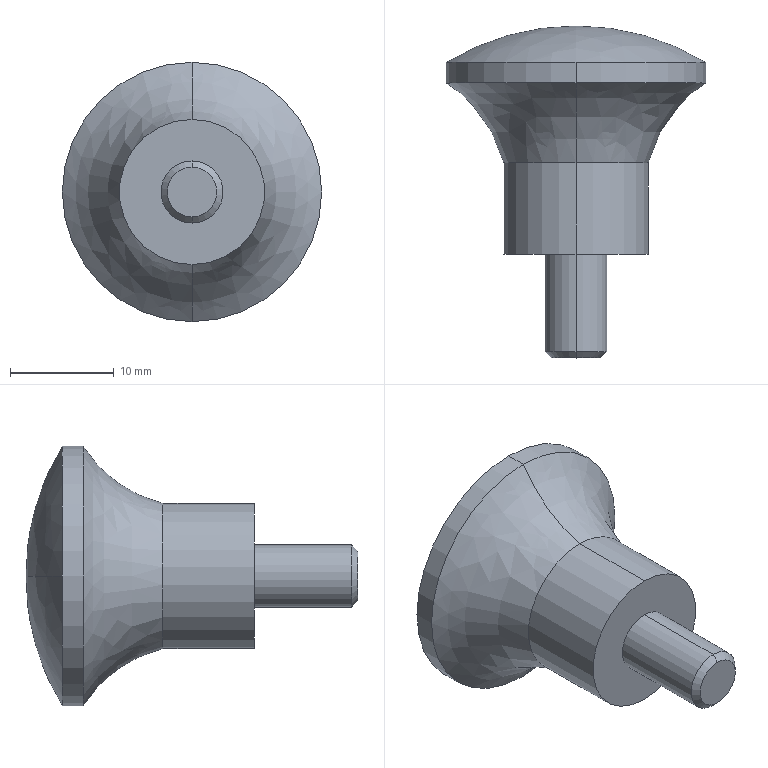Part | STEP file | 0217_011_NMM6-25 | 1 solid | 14 faces | box 25 x 32 x 25 mm | volume 5504 mm3 | cylinder 6 | spline 4 | cone 2 | plane 2 | commonest cylinder face diameters 6 x2 14 x2 25 x2
STEP:
#1=CARTESIAN_POINT('',(0.,0.,0.));
#2=DIRECTION('',(0.,0.,1.));
#3=DIRECTION('',(1.,0.,0.));
#4=AXIS2_PLACEMENT_3D('',#1,#2,#3);
#5=CARTESIAN_POINT('',(0.,18.488,12.5));
#6=VERTEX_POINT('',#5);
#7=CARTESIAN_POINT('',(12.5,18.488,0.));
#8=VERTEX_POINT('',#7);
#9=CARTESIAN_POINT('',(0.,18.488,0.));
#10=DIRECTION('',(0.,1.,0.));
#11=DIRECTION('',(0.,0.,-1.));
#12=AXIS2_PLACEMENT_3D('',#9,#10,#11);
#13=CIRCLE('',#12,12.5);
#14=CARTESIAN_POINT('',(12.634,18.405,0.));
#15=CARTESIAN_POINT('',(12.634,18.405,3.797));
#16=CARTESIAN_POINT('',(12.634,17.372,7.45));
#17=CARTESIAN_POINT('',(12.634,15.384,10.685));
#18=CARTESIAN_POINT('',(4.679,23.331,0.));
#19=CARTESIAN_POINT('',(4.679,23.331,4.713));
#20=CARTESIAN_POINT('',(4.679,22.049,9.249));
#21=CARTESIAN_POINT('',(4.679,19.581,13.264));
#22=CARTESIAN_POINT('',(-4.679,23.331,0.));
#23=CARTESIAN_POINT('',(-4.679,23.331,4.713));
#24=CARTESIAN_POINT('',(-4.679,22.049,9.249));
#25=CARTESIAN_POINT('',(-4.679,19.581,13.264));
#26=CARTESIAN_POINT('',(-12.634,18.405,0.));
#27=CARTESIAN_POINT('',(-12.634,18.405,3.797));
#28=CARTESIAN_POINT('',(-12.634,17.372,7.45));
#29=CARTESIAN_POINT('',(-12.634,15.384,10.685));
#30=(BOUNDED_SURFACE()B_SPLINE_SURFACE(3,3,((#14,#15,#16,#17),(#18,#19,#20,#21),(#22,#23,#24,#25),(#26,#27,#28,#29)),.UNSPECIFIED.,.F.,.F.,.F.)B_SPLINE_SURFACE_WITH_KNOTS((4,4),(4,4),(0.,1.),(0.,1.),.PIECEWISE_BEZIER_KNOTS.)GEOMETRIC_REPRESENTATION_ITEM()RATIONAL_B_SPLINE_SURFACE(((1.,0.9748,0.9748,1.),(0.9001,0.8775,0.8775,0.9001),(0.9001,0.8775,0.8775,0.9001),(1.,0.9748,0.9748,1.)))REPRESENTATION_ITEM('')SURFACE());
#31=CARTESIAN_POINT('',(0.5,0.994));
#32=CARTESIAN_POINT('',(0.4891,0.994));
#33=CARTESIAN_POINT('',(0.4673,0.9926));
#34=CARTESIAN_POINT('',(0.4347,0.9863));
#35=CARTESIAN_POINT('',(0.4024,0.9759));
#36=CARTESIAN_POINT('',(0.3703,0.9613));
#37=CARTESIAN_POINT('',(0.3386,0.9424));
#38=CARTESIAN_POINT('',(0.3075,0.9193));
#39=CARTESIAN_POINT('',(0.277,0.8918));
#40=CARTESIAN_POINT('',(0.2473,0.8601));
#41=CARTESIAN_POINT('',(0.2185,0.8239));
#42=CARTESIAN_POINT('',(0.1908,0.7835));
#43=CARTESIAN_POINT('',(0.1644,0.7386));
#44=CARTESIAN_POINT('',(0.1393,0.6894));
#45=CARTESIAN_POINT('',(0.1159,0.6359));
#46=CARTESIAN_POINT('',(0.09419,0.5783));
#47=CARTESIAN_POINT('',(0.07447,0.5167));
#48=CARTESIAN_POINT('',(0.05692,0.4513));
#49=CARTESIAN_POINT('',(0.04169,0.3824));
#50=CARTESIAN_POINT('',(0.02897,0.3104));
#51=CARTESIAN_POINT('',(0.01891,0.2356));
#52=CARTESIAN_POINT('',(0.01163,0.1586));
#53=CARTESIAN_POINT('',(0.007223,0.07989));
#54=CARTESIAN_POINT('',(0.006235,0.02669));
#55=CARTESIAN_POINT('',(0.006238,0.));
#56=B_SPLINE_CURVE_WITH_KNOTS('',3,(#31,#32,#33,#34,#35,#36,#37,#38,#39,#40,#41,#42,#43,#44,#45,#46,#47,#48,#49,#50,#51,#52,#53,#54,#55),.UNSPECIFIED.,.F.,.F.,(4,1,1,1,1,1,1,1,1,1,1,1,1,1,1,1,1,1,1,1,1,1,4),(3.142,3.213,3.284,3.356,3.427,3.499,3.57,3.641,3.713,3.784,3.856,3.927,3.998,4.07,4.141,4.213,4.284,4.355,4.427,4.498,4.57,4.641,4.712),.QUASI_UNIFORM_KNOTS.);
#57=(GEOMETRIC_REPRESENTATION_CONTEXT(2)PARAMETRIC_REPRESENTATION_CONTEXT()REPRESENTATION_CONTEXT('',''));
#58=DEFINITIONAL_REPRESENTATION('',(#56),#57);
#59=PCURVE('',#30,#58);
#60=CARTESIAN_POINT('',(0.,17.494,0.));
#61=DIRECTION('',(0.,-1.,0.));
#62=DIRECTION('',(0.,0.,-1.));
#63=AXIS2_PLACEMENT_3D('',#60,#61,#62);
#64=CYLINDRICAL_SURFACE('',#63,12.5);
#65=CARTESIAN_POINT('',(6.283,-0.9939));
#66=DIRECTION('',(-1.,0.));
#67=VECTOR('',#66,1.);
#68=LINE('',#65,#67);
#69=(GEOMETRIC_REPRESENTATION_CONTEXT(2)PARAMETRIC_REPRESENTATION_CONTEXT()REPRESENTATION_CONTEXT('',''));
#70=DEFINITIONAL_REPRESENTATION('',(#68),#69);
#71=PCURVE('',#64,#70);
#72=SURFACE_CURVE('',#13,(#59,#71),.PCURVE_S1.);
#73=EDGE_CURVE('',#6,#8,#72,.T.);
#74=ORIENTED_EDGE('',*,*,#73,.T.);
#75=CARTESIAN_POINT('',(-12.5,18.488,0.));
#76=VERTEX_POINT('',#75);
#77=CARTESIAN_POINT('',(0.,-2.,0.));
#78=DIRECTION('',(0.,0.,1.));
#79=DIRECTION('',(1.,0.,0.));
#80=AXIS2_PLACEMENT_3D('',#77,#78,#79);
#81=CIRCLE('',#80,24.);
#82=CARTESIAN_POINT('',(0.006238,0.));
#83=CARTESIAN_POINT('',(0.02198,0.));
#84=CARTESIAN_POINT('',(0.05323,0.));
#85=CARTESIAN_POINT('',(0.09953,0.));
#86=CARTESIAN_POINT('',(0.1453,0.));
#87=CARTESIAN_POINT('',(0.1906,0.));
#88=CARTESIAN_POINT('',(0.2355,0.));
#89=CARTESIAN_POINT('',(0.2801,0.));
#90=CARTESIAN_POINT('',(0.3244,0.));
#91=CARTESIAN_POINT('',(0.3685,0.));
#92=CARTESIAN_POINT('',(0.4124,0.));
#93=CARTESIAN_POINT('',(0.4562,0.));
#94=CARTESIAN_POINT('',(0.5,0.));
#95=CARTESIAN_POINT('',(0.5438,0.));
#96=CARTESIAN_POINT('',(0.5876,0.));
#97=CARTESIAN_POINT('',(0.6315,0.));
#98=CARTESIAN_POINT('',(0.6756,0.));
#99=CARTESIAN_POINT('',(0.7199,0.));
#100=CARTESIAN_POINT('',(0.7645,0.));
#101=CARTESIAN_POINT('',(0.8094,0.));
#102=CARTESIAN_POINT('',(0.8547,0.));
#103=CARTESIAN_POINT('',(0.9005,0.));
#104=CARTESIAN_POINT('',(0.9468,0.));
#105=CARTESIAN_POINT('',(0.978,0.));
#106=CARTESIAN_POINT('',(0.9938,0.));
#107=B_SPLINE_CURVE_WITH_KNOTS('',3,(#82,#83,#84,#85,#86,#87,#88,#89,#90,#91,#92,#93,#94,#95,#96,#97,#98,#99,#100,#101,#102,#103,#104,#105,#106),.UNSPECIFIED.,.F.,.F.,(4,1,1,1,1,1,1,1,1,1,1,1,1,1,1,1,1,1,1,1,1,1,4),(1.023,1.073,1.123,1.172,1.222,1.272,1.322,1.372,1.421,1.471,1.521,1.571,1.621,1.67,1.72,1.77,1.82,1.87,1.919,1.969,2.019,2.069,2.119),.QUASI_UNIFORM_KNOTS.);
#108=(GEOMETRIC_REPRESENTATION_CONTEXT(2)PARAMETRIC_REPRESENTATION_CONTEXT()REPRESENTATION_CONTEXT('',''));
#109=DEFINITIONAL_REPRESENTATION('',(#107),#108);
#110=PCURVE('',#30,#109);
#111=CARTESIAN_POINT('',(12.634,15.384,-10.685));
#112=CARTESIAN_POINT('',(12.634,17.372,-7.45));
#113=CARTESIAN_POINT('',(12.634,18.405,-3.797));
#114=CARTESIAN_POINT('',(12.634,18.405,0.));
#115=CARTESIAN_POINT('',(4.679,19.581,-13.264));
#116=CARTESIAN_POINT('',(4.679,22.049,-9.249));
#117=CARTESIAN_POINT('',(4.679,23.331,-4.713));
#118=CARTESIAN_POINT('',(4.679,23.331,0.));
#119=CARTESIAN_POINT('',(-4.679,19.581,-13.264));
#120=CARTESIAN_POINT('',(-4.679,22.049,-9.249));
#121=CARTESIAN_POINT('',(-4.679,23.331,-4.713));
#122=CARTESIAN_POINT('',(-4.679,23.331,0.));
#123=CARTESIAN_POINT('',(-12.634,15.384,-10.685));
#124=CARTESIAN_POINT('',(-12.634,17.372,-7.45));
#125=CARTESIAN_POINT('',(-12.634,18.405,-3.797));
#126=CARTESIAN_POINT('',(-12.634,18.405,0.));
#127=(BOUNDED_SURFACE()B_SPLINE_SURFACE(3,3,((#111,#112,#113,#114),(#115,#116,#117,#118),(#119,#120,#121,#122),(#123,#124,#125,#126)),.UNSPECIFIED.,.F.,.F.,.F.)B_SPLINE_SURFACE_WITH_KNOTS((4,4),(4,4),(0.,1.),(0.,1.),.PIECEWISE_BEZIER_KNOTS.)GEOMETRIC_REPRESENTATION_ITEM()RATIONAL_B_SPLINE_SURFACE(((1.,0.9748,0.9748,1.),(0.9001,0.8775,0.8775,0.9001),(0.9001,0.8775,0.8775,0.9001),(1.,0.9748,0.9748,1.)))REPRESENTATION_ITEM('')SURFACE());
#128=CARTESIAN_POINT('',(0.006238,1.));
#129=CARTESIAN_POINT('',(0.02198,1.));
#130=CARTESIAN_POINT('',(0.05323,1.));
#131=CARTESIAN_POINT('',(0.09953,1.));
#132=CARTESIAN_POINT('',(0.1453,1.));
#133=CARTESIAN_POINT('',(0.1906,1.));
#134=CARTESIAN_POINT('',(0.2355,1.));
#135=CARTESIAN_POINT('',(0.2801,1.));
#136=CARTESIAN_POINT('',(0.3244,1.));
#137=CARTESIAN_POINT('',(0.3685,1.));
#138=CARTESIAN_POINT('',(0.4124,1.));
#139=CARTESIAN_POINT('',(0.4562,1.));
#140=CARTESIAN_POINT('',(0.5,1.));
#141=CARTESIAN_POINT('',(0.5438,1.));
#142=CARTESIAN_POINT('',(0.5876,1.));
#143=CARTESIAN_POINT('',(0.6315,1.));
#144=CARTESIAN_POINT('',(0.6756,1.));
#145=CARTESIAN_POINT('',(0.7199,1.));
#146=CARTESIAN_POINT('',(0.7645,1.));
#147=CARTESIAN_POINT('',(0.8094,1.));
#148=CARTESIAN_POINT('',(0.8547,1.));
#149=CARTESIAN_POINT('',(0.9005,1.));
#150=CARTESIAN_POINT('',(0.9468,1.));
#151=CARTESIAN_POINT('',(0.978,1.));
#152=CARTESIAN_POINT('',(0.9938,1.));
#153=B_SPLINE_CURVE_WITH_KNOTS('',3,(#128,#129,#130,#131,#132,#133,#134,#135,#136,#137,#138,#139,#140,#141,#142,#143,#144,#145,#146,#147,#148,#149,#150,#151,#152),.UNSPECIFIED.,.F.,.F.,(4,1,1,1,1,1,1,1,1,1,1,1,1,1,1,1,1,1,1,1,1,1,4),(1.023,1.073,1.123,1.172,1.222,1.272,1.322,1.372,1.421,1.471,1.521,1.571,1.621,1.67,1.72,1.77,1.82,1.87,1.919,1.969,2.019,2.069,2.119),.QUASI_UNIFORM_KNOTS.);
#154=(GEOMETRIC_REPRESENTATION_CONTEXT(2)PARAMETRIC_REPRESENTATION_CONTEXT()REPRESENTATION_CONTEXT('',''));
#155=DEFINITIONAL_REPRESENTATION('',(#153),#154);
#156=PCURVE('',#127,#155);
#157=SURFACE_CURVE('',#81,(#110,#156),.PCURVE_S1.);
#158=EDGE_CURVE('',#8,#76,#157,.T.);
#159=ORIENTED_EDGE('',*,*,#158,.T.);
#160=CARTESIAN_POINT('',(0.,18.488,0.));
#161=DIRECTION('',(0.,1.,0.));
#162=DIRECTION('',(0.,0.,-1.));
#163=AXIS2_PLACEMENT_3D('',#160,#161,#162);
#164=CIRCLE('',#163,12.5);
#165=CARTESIAN_POINT('',(0.9938,0.));
#166=CARTESIAN_POINT('',(0.9938,0.02669));
#167=CARTESIAN_POINT('',(0.9928,0.07989));
#168=CARTESIAN_POINT('',(0.9884,0.1586));
#169=CARTESIAN_POINT('',(0.9811,0.2356));
#170=CARTESIAN_POINT('',(0.971,0.3104));
#171=CARTESIAN_POINT('',(0.9583,0.3824));
#172=CARTESIAN_POINT('',(0.9431,0.4513));
#173=CARTESIAN_POINT('',(0.9255,0.5167));
#174=CARTESIAN_POINT('',(0.9058,0.5783));
#175=CARTESIAN_POINT('',(0.8841,0.6359));
#176=CARTESIAN_POINT('',(0.8607,0.6894));
#177=CARTESIAN_POINT('',(0.8356,0.7386));
#178=CARTESIAN_POINT('',(0.8092,0.7835));
#179=CARTESIAN_POINT('',(0.7815,0.8239));
#180=CARTESIAN_POINT('',(0.7527,0.8601));
#181=CARTESIAN_POINT('',(0.723,0.8918));
#182=CARTESIAN_POINT('',(0.6925,0.9193));
#183=CARTESIAN_POINT('',(0.6614,0.9424));
#184=CARTESIAN_POINT('',(0.6297,0.9613));
#185=CARTESIAN_POINT('',(0.5976,0.9759));
#186=CARTESIAN_POINT('',(0.5653,0.9863));
#187=CARTESIAN_POINT('',(0.5327,0.9926));
#188=CARTESIAN_POINT('',(0.5109,0.994));
#189=CARTESIAN_POINT('',(0.5,0.994));
#190=B_SPLINE_CURVE_WITH_KNOTS('',3,(#165,#166,#167,#168,#169,#170,#171,#172,#173,#174,#175,#176,#177,#178,#179,#180,#181,#182,#183,#184,#185,#186,#187,#188,#189),.UNSPECIFIED.,.F.,.F.,(4,1,1,1,1,1,1,1,1,1,1,1,1,1,1,1,1,1,1,1,1,1,4),(1.571,1.642,1.714,1.785,1.856,1.928,1.999,2.071,2.142,2.213,2.285,2.356,2.428,2.499,2.57,2.642,2.713,2.785,2.856,2.927,2.999,3.07,3.142),.QUASI_UNIFORM_KNOTS.);
#191=(GEOMETRIC_REPRESENTATION_CONTEXT(2)PARAMETRIC_REPRESENTATION_CONTEXT()REPRESENTATION_CONTEXT('',''));
#192=DEFINITIONAL_REPRESENTATION('',(#190),#191);
#193=PCURVE('',#30,#192);
#194=CARTESIAN_POINT('',(0.,17.494,0.));
#195=DIRECTION('',(0.,-1.,0.));
#196=DIRECTION('',(0.,0.,-1.));
#197=AXIS2_PLACEMENT_3D('',#194,#195,#196);
#198=CYLINDRICAL_SURFACE('',#197,12.5);
#199=CARTESIAN_POINT('',(6.283,-0.9939));
#200=DIRECTION('',(-1.,0.));
#201=VECTOR('',#200,1.);
#202=LINE('',#199,#201);
#203=(GEOMETRIC_REPRESENTATION_CONTEXT(2)PARAMETRIC_REPRESENTATION_CONTEXT()REPRESENTATION_CONTEXT('',''));
#204=DEFINITIONAL_REPRESENTATION('',(#202),#203);
#205=PCURVE('',#198,#204);
#206=SURFACE_CURVE('',#164,(#193,#205),.PCURVE_S1.);
#207=EDGE_CURVE('',#76,#6,#206,.T.);
#208=ORIENTED_EDGE('',*,*,#207,.T.);
#209=EDGE_LOOP('',(#74,#159,#208));
#210=FACE_BOUND('',#209,.T.);
#211=ADVANCED_FACE('',(#210),#30,.T.);
#212=CARTESIAN_POINT('',(0.,8.8,7.));
#213=VERTEX_POINT('',#212);
#214=CARTESIAN_POINT('',(0.,16.5,12.5));
#215=VERTEX_POINT('',#214);
#216=CARTESIAN_POINT('',(0.,5.925,19.165));
#217=DIRECTION('',(1.,0.,0.));
#218=DIRECTION('',(0.,0.,1.));
#219=AXIS2_PLACEMENT_3D('',#216,#217,#218);
#220=CIRCLE('',#219,12.5);
#221=CARTESIAN_POINT('',(0.,8.8,7.));
#222=CARTESIAN_POINT('',(14.,8.8,7.));
#223=CARTESIAN_POINT('',(14.,8.8,-7.));
#224=CARTESIAN_POINT('',(0.,8.8,-7.));
#225=CARTESIAN_POINT('',(0.,12.03,7.763));
#226=CARTESIAN_POINT('',(15.527,12.03,7.763));
#227=CARTESIAN_POINT('',(15.527,12.03,-7.763));
#228=CARTESIAN_POINT('',(0.,12.03,-7.763));
#229=CARTESIAN_POINT('',(0.,14.73,9.692));
#230=CARTESIAN_POINT('',(19.385,14.73,9.692));
#231=CARTESIAN_POINT('',(19.385,14.73,-9.692));
#232=CARTESIAN_POINT('',(0.,14.73,-9.692));
#233=CARTESIAN_POINT('',(0.,16.5,12.5));
#234=CARTESIAN_POINT('',(25.,16.5,12.5));
#235=CARTESIAN_POINT('',(25.,16.5,-12.5));
#236=CARTESIAN_POINT('',(0.,16.5,-12.5));
#237=(BOUNDED_SURFACE()B_SPLINE_SURFACE(3,3,((#221,#222,#223,#224),(#225,#226,#227,#228),(#229,#230,#231,#232),(#233,#234,#235,#236)),.UNSPECIFIED.,.F.,.F.,.F.)B_SPLINE_SURFACE_WITH_KNOTS((4,4),(4,4),(0.,1.),(0.,1.),.PIECEWISE_BEZIER_KNOTS.)GEOMETRIC_REPRESENTATION_ITEM()RATIONAL_B_SPLINE_SURFACE(((1.,0.3333,0.3333,1.),(0.9504,0.3168,0.3168,0.9504),(0.9504,0.3168,0.3168,0.9504),(1.,0.3333,0.3333,1.)))REPRESENTATION_ITEM('')SURFACE());
#238=CARTESIAN_POINT('',(0.,0.));
#239=CARTESIAN_POINT('',(0.01554,0.));
#240=CARTESIAN_POINT('',(0.04651,0.));
#241=CARTESIAN_POINT('',(0.09267,0.));
#242=CARTESIAN_POINT('',(0.1386,0.));
#243=CARTESIAN_POINT('',(0.1842,0.));
#244=CARTESIAN_POINT('',(0.2297,0.));
#245=CARTESIAN_POINT('',(0.275,0.));
#246=CARTESIAN_POINT('',(0.3202,0.));
#247=CARTESIAN_POINT('',(0.3652,0.));
#248=CARTESIAN_POINT('',(0.4102,0.));
#249=CARTESIAN_POINT('',(0.4551,0.));
#250=CARTESIAN_POINT('',(0.5,0.));
#251=CARTESIAN_POINT('',(0.5449,0.));
#252=CARTESIAN_POINT('',(0.5898,0.));
#253=CARTESIAN_POINT('',(0.6348,0.));
#254=CARTESIAN_POINT('',(0.6798,0.));
#255=CARTESIAN_POINT('',(0.725,0.));
#256=CARTESIAN_POINT('',(0.7703,0.));
#257=CARTESIAN_POINT('',(0.8158,0.));
#258=CARTESIAN_POINT('',(0.8614,0.));
#259=CARTESIAN_POINT('',(0.9073,0.));
#260=CARTESIAN_POINT('',(0.9535,0.));
#261=CARTESIAN_POINT('',(0.9845,0.));
#262=CARTESIAN_POINT('',(1.,0.));
#263=B_SPLINE_CURVE_WITH_KNOTS('',3,(#238,#239,#240,#241,#242,#243,#244,#245,#246,#247,#248,#249,#250,#251,#252,#253,#254,#255,#256,#257,#258,#259,#260,#261,#262),.UNSPECIFIED.,.F.,.F.,(4,1,1,1,1,1,1,1,1,1,1,1,1,1,1,1,1,1,1,1,1,1,4),(3.374,3.409,3.444,3.48,3.515,3.55,3.585,3.621,3.656,3.691,3.727,3.762,3.797,3.832,3.868,3.903,3.938,3.974,4.009,4.044,4.079,4.115,4.15),.QUASI_UNIFORM_KNOTS.);
#264=(GEOMETRIC_REPRESENTATION_CONTEXT(2)PARAMETRIC_REPRESENTATION_CONTEXT()REPRESENTATION_CONTEXT('',''));
#265=DEFINITIONAL_REPRESENTATION('',(#263),#264);
#266=PCURVE('',#237,#265);
#267=CARTESIAN_POINT('',(0.,8.8,-7.));
#268=CARTESIAN_POINT('',(-14.,8.8,-7.));
#269=CARTESIAN_POINT('',(-14.,8.8,7.));
#270=CARTESIAN_POINT('',(0.,8.8,7.));
#271=CARTESIAN_POINT('',(0.,12.03,-7.763));
#272=CARTESIAN_POINT('',(-15.527,12.03,-7.763));
#273=CARTESIAN_POINT('',(-15.527,12.03,7.763));
#274=CARTESIAN_POINT('',(0.,12.03,7.763));
#275=CARTESIAN_POINT('',(0.,14.73,-9.692));
#276=CARTESIAN_POINT('',(-19.385,14.73,-9.692));
#277=CARTESIAN_POINT('',(-19.385,14.73,9.692));
#278=CARTESIAN_POINT('',(0.,14.73,9.692));
#279=CARTESIAN_POINT('',(0.,16.5,-12.5));
#280=CARTESIAN_POINT('',(-25.,16.5,-12.5));
#281=CARTESIAN_POINT('',(-25.,16.5,12.5));
#282=CARTESIAN_POINT('',(0.,16.5,12.5));
#283=(BOUNDED_SURFACE()B_SPLINE_SURFACE(3,3,((#267,#268,#269,#270),(#271,#272,#273,#274),(#275,#276,#277,#278),(#279,#280,#281,#282)),.UNSPECIFIED.,.F.,.F.,.F.)B_SPLINE_SURFACE_WITH_KNOTS((4,4),(4,4),(0.,1.),(0.,1.),.PIECEWISE_BEZIER_KNOTS.)GEOMETRIC_REPRESENTATION_ITEM()RATIONAL_B_SPLINE_SURFACE(((1.,0.3333,0.3333,1.),(0.9504,0.3168,0.3168,0.9504),(0.9504,0.3168,0.3168,0.9504),(1.,0.3333,0.3333,1.)))REPRESENTATION_ITEM('')SURFACE());
#284=CARTESIAN_POINT('',(0.,1.));
#285=CARTESIAN_POINT('',(0.01554,1.));
#286=CARTESIAN_POINT('',(0.04651,1.));
#287=CARTESIAN_POINT('',(0.09267,1.));
#288=CARTESIAN_POINT('',(0.1386,1.));
#289=CARTESIAN_POINT('',(0.1842,1.));
#290=CARTESIAN_POINT('',(0.2297,1.));
#291=CARTESIAN_POINT('',(0.275,1.));
#292=CARTESIAN_POINT('',(0.3202,1.));
#293=CARTESIAN_POINT('',(0.3652,1.));
#294=CARTESIAN_POINT('',(0.4102,1.));
#295=CARTESIAN_POINT('',(0.4551,1.));
#296=CARTESIAN_POINT('',(0.5,1.));
#297=CARTESIAN_POINT('',(0.5449,1.));
#298=CARTESIAN_POINT('',(0.5898,1.));
#299=CARTESIAN_POINT('',(0.6348,1.));
#300=CARTESIAN_POINT('',(0.6798,1.));
#301=CARTESIAN_POINT('',(0.725,1.));
#302=CARTESIAN_POINT('',(0.7703,1.));
#303=CARTESIAN_POINT('',(0.8158,1.));
#304=CARTESIAN_POINT('',(0.8614,1.));
#305=CARTESIAN_POINT('',(0.9073,1.));
#306=CARTESIAN_POINT('',(0.9535,1.));
#307=CARTESIAN_POINT('',(0.9845,1.));
#308=CARTESIAN_POINT('',(1.,1.));
#309=B_SPLINE_CURVE_WITH_KNOTS('',3,(#284,#285,#286,#287,#288,#289,#290,#291,#292,#293,#294,#295,#296,#297,#298,#299,#300,#301,#302,#303,#304,#305,#306,#307,#308),.UNSPECIFIED.,.F.,.F.,(4,1,1,1,1,1,1,1,1,1,1,1,1,1,1,1,1,1,1,1,1,1,4),(3.374,3.409,3.444,3.48,3.515,3.55,3.585,3.621,3.656,3.691,3.727,3.762,3.797,3.832,3.868,3.903,3.938,3.974,4.009,4.044,4.079,4.115,4.15),.QUASI_UNIFORM_KNOTS.);
#310=(GEOMETRIC_REPRESENTATION_CONTEXT(2)PARAMETRIC_REPRESENTATION_CONTEXT()REPRESENTATION_CONTEXT('',''));
#311=DEFINITIONAL_REPRESENTATION('',(#309),#310);
#312=PCURVE('',#283,#311);
#313=SURFACE_CURVE('',#220,(#266,#312),.PCURVE_S1.);
#314=EDGE_CURVE('',#213,#215,#313,.T.);
#315=ORIENTED_EDGE('',*,*,#314,.T.);
#316=CARTESIAN_POINT('',(0.,16.5,-12.5));
#317=VERTEX_POINT('',#316);
#318=CARTESIAN_POINT('',(0.,16.5,0.));
#319=DIRECTION('',(0.,1.,0.));
#320=DIRECTION('',(0.,0.,-1.));
#321=AXIS2_PLACEMENT_3D('',#318,#319,#320);
#322=CIRCLE('',#321,12.5);
#323=CARTESIAN_POINT('',(1.,0.));
#324=CARTESIAN_POINT('',(1.,0.02375));
#325=CARTESIAN_POINT('',(1.,0.06805));
#326=CARTESIAN_POINT('',(1.,0.1267));
#327=CARTESIAN_POINT('',(1.,0.1794));
#328=CARTESIAN_POINT('',(1.,0.2276));
#329=CARTESIAN_POINT('',(1.,0.2721));
#330=CARTESIAN_POINT('',(1.,0.3139));
#331=CARTESIAN_POINT('',(1.,0.3535));
#332=CARTESIAN_POINT('',(1.,0.3914));
#333=CARTESIAN_POINT('',(1.,0.4282));
#334=CARTESIAN_POINT('',(1.,0.4643));
#335=CARTESIAN_POINT('',(1.,0.5));
#336=CARTESIAN_POINT('',(1.,0.5357));
#337=CARTESIAN_POINT('',(1.,0.5718));
#338=CARTESIAN_POINT('',(1.,0.6086));
#339=CARTESIAN_POINT('',(1.,0.6465));
#340=CARTESIAN_POINT('',(1.,0.6861));
#341=CARTESIAN_POINT('',(1.,0.7279));
#342=CARTESIAN_POINT('',(1.,0.7724));
#343=CARTESIAN_POINT('',(1.,0.8206));
#344=CARTESIAN_POINT('',(1.,0.8733));
#345=CARTESIAN_POINT('',(1.,0.9319));
#346=CARTESIAN_POINT('',(1.,0.9763));
#347=CARTESIAN_POINT('',(1.,1.));
#348=B_SPLINE_CURVE_WITH_KNOTS('',3,(#323,#324,#325,#326,#327,#328,#329,#330,#331,#332,#333,#334,#335,#336,#337,#338,#339,#340,#341,#342,#343,#344,#345,#346,#347),.UNSPECIFIED.,.F.,.F.,(4,1,1,1,1,1,1,1,1,1,1,1,1,1,1,1,1,1,1,1,1,1,4),(3.142,3.284,3.427,3.57,3.713,3.856,3.998,4.141,4.284,4.427,4.57,4.712,4.855,4.998,5.141,5.284,5.426,5.569,5.712,5.855,5.998,6.14,6.283),.QUASI_UNIFORM_KNOTS.);
#349=(GEOMETRIC_REPRESENTATION_CONTEXT(2)PARAMETRIC_REPRESENTATION_CONTEXT()REPRESENTATION_CONTEXT('',''));
#350=DEFINITIONAL_REPRESENTATION('',(#348),#349);
#351=PCURVE('',#237,#350);
#352=CARTESIAN_POINT('',(6.283,0.9939));
#353=DIRECTION('',(-1.,0.));
#354=VECTOR('',#353,1.);
#355=LINE('',#352,#354);
#356=(GEOMETRIC_REPRESENTATION_CONTEXT(2)PARAMETRIC_REPRESENTATION_CONTEXT()REPRESENTATION_CONTEXT('',''));
#357=DEFINITIONAL_REPRESENTATION('',(#355),#356);
#358=PCURVE('',#64,#357);
#359=SURFACE_CURVE('',#322,(#351,#358),.PCURVE_S1.);
#360=EDGE_CURVE('',#215,#317,#359,.T.);
#361=ORIENTED_EDGE('',*,*,#360,.T.);
#362=CARTESIAN_POINT('',(0.,8.8,-7.));
#363=VERTEX_POINT('',#362);
#364=CARTESIAN_POINT('',(0.,5.925,-19.165));
#365=DIRECTION('',(-1.,0.,0.));
#366=DIRECTION('',(0.,0.,-1.));
#367=AXIS2_PLACEMENT_3D('',#364,#365,#366);
#368=CIRCLE('',#367,12.5);
#369=CARTESIAN_POINT('',(0.,1.));
#370=CARTESIAN_POINT('',(0.01554,1.));
#371=CARTESIAN_POINT('',(0.04651,1.));
#372=CARTESIAN_POINT('',(0.09267,1.));
#373=CARTESIAN_POINT('',(0.1386,1.));
#374=CARTESIAN_POINT('',(0.1842,1.));
#375=CARTESIAN_POINT('',(0.2297,1.));
#376=CARTESIAN_POINT('',(0.275,1.));
#377=CARTESIAN_POINT('',(0.3202,1.));
#378=CARTESIAN_POINT('',(0.3652,1.));
#379=CARTESIAN_POINT('',(0.4102,1.));
#380=CARTESIAN_POINT('',(0.4551,1.));
#381=CARTESIAN_POINT('',(0.5,1.));
#382=CARTESIAN_POINT('',(0.5449,1.));
#383=CARTESIAN_POINT('',(0.5898,1.));
#384=CARTESIAN_POINT('',(0.6348,1.));
#385=CARTESIAN_POINT('',(0.6798,1.));
#386=CARTESIAN_POINT('',(0.725,1.));
#387=CARTESIAN_POINT('',(0.7703,1.));
#388=CARTESIAN_POINT('',(0.8158,1.));
#389=CARTESIAN_POINT('',(0.8614,1.));
#390=CARTESIAN_POINT('',(0.9073,1.));
#391=CARTESIAN_POINT('',(0.9535,1.));
#392=CARTESIAN_POINT('',(0.9845,1.));
#393=CARTESIAN_POINT('',(1.,1.));
#394=B_SPLINE_CURVE_WITH_KNOTS('',3,(#369,#370,#371,#372,#373,#374,#375,#376,#377,#378,#379,#380,#381,#382,#383,#384,#385,#386,#387,#388,#389,#390,#391,#392,#393),.UNSPECIFIED.,.F.,.F.,(4,1,1,1,1,1,1,1,1,1,1,1,1,1,1,1,1,1,1,1,1,1,4),(3.374,3.409,3.444,3.48,3.515,3.55,3.585,3.621,3.656,3.691,3.727,3.762,3.797,3.832,3.868,3.903,3.938,3.974,4.009,4.044,4.079,4.115,4.15),.QUASI_UNIFORM_KNOTS.);
#395=(GEOMETRIC_REPRESENTATION_CONTEXT(2)PARAMETRIC_REPRESENTATION_CONTEXT()REPRESENTATION_CONTEXT('',''));
#396=DEFINITIONAL_REPRESENTATION('',(#394),#395);
#397=PCURVE('',#237,#396);
#398=CARTESIAN_POINT('',(0.,0.));
#399=CARTESIAN_POINT('',(0.01554,0.));
#400=CARTESIAN_POINT('',(0.04651,0.));
#401=CARTESIAN_POINT('',(0.09267,0.));
#402=CARTESIAN_POINT('',(0.1386,0.));
#403=CARTESIAN_POINT('',(0.1842,0.));
#404=CARTESIAN_POINT('',(0.2297,0.));
#405=CARTESIAN_POINT('',(0.275,0.));
#406=CARTESIAN_POINT('',(0.3202,0.));
#407=CARTESIAN_POINT('',(0.3652,0.));
#408=CARTESIAN_POINT('',(0.4102,0.));
#409=CARTESIAN_POINT('',(0.4551,0.));
#410=CARTESIAN_POINT('',(0.5,0.));
#411=CARTESIAN_POINT('',(0.5449,0.));
#412=CARTESIAN_POINT('',(0.5898,0.));
#413=CARTESIAN_POINT('',(0.6348,0.));
#414=CARTESIAN_POINT('',(0.6798,0.));
#415=CARTESIAN_POINT('',(0.725,0.));
#416=CARTESIAN_POINT('',(0.7703,0.));
#417=CARTESIAN_POINT('',(0.8158,0.));
#418=CARTESIAN_POINT('',(0.8614,0.));
#419=CARTESIAN_POINT('',(0.9073,0.));
#420=CARTESIAN_POINT('',(0.9535,0.));
#421=CARTESIAN_POINT('',(0.9845,0.));
#422=CARTESIAN_POINT('',(1.,0.));
#423=B_SPLINE_CURVE_WITH_KNOTS('',3,(#398,#399,#400,#401,#402,#403,#404,#405,#406,#407,#408,#409,#410,#411,#412,#413,#414,#415,#416,#417,#418,#419,#420,#421,#422),.UNSPECIFIED.,.F.,.F.,(4,1,1,1,1,1,1,1,1,1,1,1,1,1,1,1,1,1,1,1,1,1,4),(3.374,3.409,3.444,3.48,3.515,3.55,3.585,3.621,3.656,3.691,3.727,3.762,3.797,3.832,3.868,3.903,3.938,3.974,4.009,4.044,4.079,4.115,4.15),.QUASI_UNIFORM_KNOTS.);
#424=(GEOMETRIC_REPRESENTATION_CONTEXT(2)PARAMETRIC_REPRESENTATION_CONTEXT()REPRESENTATION_CONTEXT('',''));
#425=DEFINITIONAL_REPRESENTATION('',(#423),#424);
#426=PCURVE('',#283,#425);
#427=SURFACE_CURVE('',#368,(#397,#426),.PCURVE_S1.);
#428=EDGE_CURVE('',#363,#317,#427,.T.);
#429=ORIENTED_EDGE('',*,*,#428,.F.);
#430=CARTESIAN_POINT('',(0.,8.8,0.));
#431=DIRECTION('',(0.,-1.,0.));
#432=DIRECTION('',(0.,0.,1.));
#433=AXIS2_PLACEMENT_3D('',#430,#431,#432);
#434=CIRCLE('',#433,7.);
#435=CARTESIAN_POINT('',(0.,1.));
#436=CARTESIAN_POINT('',(0.,0.9763));
#437=CARTESIAN_POINT('',(0.,0.9319));
#438=CARTESIAN_POINT('',(0.,0.8733));
#439=CARTESIAN_POINT('',(0.,0.8206));
#440=CARTESIAN_POINT('',(0.,0.7724));
#441=CARTESIAN_POINT('',(0.,0.7279));
#442=CARTESIAN_POINT('',(0.,0.6861));
#443=CARTESIAN_POINT('',(0.,0.6465));
#444=CARTESIAN_POINT('',(0.,0.6086));
#445=CARTESIAN_POINT('',(0.,0.5718));
#446=CARTESIAN_POINT('',(0.,0.5357));
#447=CARTESIAN_POINT('',(0.,0.5));
#448=CARTESIAN_POINT('',(0.,0.4643));
#449=CARTESIAN_POINT('',(0.,0.4282));
#450=CARTESIAN_POINT('',(0.,0.3914));
#451=CARTESIAN_POINT('',(0.,0.3535));
#452=CARTESIAN_POINT('',(0.,0.3139));
#453=CARTESIAN_POINT('',(0.,0.2721));
#454=CARTESIAN_POINT('',(0.,0.2276));
#455=CARTESIAN_POINT('',(0.,0.1794));
#456=CARTESIAN_POINT('',(0.,0.1267));
#457=CARTESIAN_POINT('',(0.,0.06805));
#458=CARTESIAN_POINT('',(0.,0.02375));
#459=CARTESIAN_POINT('',(0.,0.));
#460=B_SPLINE_CURVE_WITH_KNOTS('',3,(#435,#436,#437,#438,#439,#440,#441,#442,#443,#444,#445,#446,#447,#448,#449,#450,#451,#452,#453,#454,#455,#456,#457,#458,#459),.UNSPECIFIED.,.F.,.F.,(4,1,1,1,1,1,1,1,1,1,1,1,1,1,1,1,1,1,1,1,1,1,4),(3.142,3.284,3.427,3.57,3.713,3.856,3.998,4.141,4.284,4.427,4.57,4.712,4.855,4.998,5.141,5.284,5.426,5.569,5.712,5.855,5.998,6.14,6.283),.QUASI_UNIFORM_KNOTS.);
#461=(GEOMETRIC_REPRESENTATION_CONTEXT(2)PARAMETRIC_REPRESENTATION_CONTEXT()REPRESENTATION_CONTEXT('',''));
#462=DEFINITIONAL_REPRESENTATION('',(#460),#461);
#463=PCURVE('',#237,#462);
#464=CARTESIAN_POINT('',(0.,4.4,0.));
#465=DIRECTION('',(0.,-1.,0.));
#466=DIRECTION('',(0.,0.,-1.));
#467=AXIS2_PLACEMENT_3D('',#464,#465,#466);
#468=CYLINDRICAL_SURFACE('',#467,7.);
#469=CARTESIAN_POINT('',(-3.142,-4.4));
#470=DIRECTION('',(1.,0.));
#471=VECTOR('',#470,1.);
#472=LINE('',#469,#471);
#473=(GEOMETRIC_REPRESENTATION_CONTEXT(2)PARAMETRIC_REPRESENTATION_CONTEXT()REPRESENTATION_CONTEXT('',''));
#474=DEFINITIONAL_REPRESENTATION('',(#472),#473);
#475=PCURVE('',#468,#474);
#476=SURFACE_CURVE('',#434,(#463,#475),.PCURVE_S1.);
#477=EDGE_CURVE('',#363,#213,#476,.T.);
#478=ORIENTED_EDGE('',*,*,#477,.T.);
#479=EDGE_LOOP('',(#315,#361,#429,#478));
#480=FACE_BOUND('',#479,.F.);
#481=ADVANCED_FACE('',(#480),#237,.F.);
#482=ORIENTED_EDGE('',*,*,#73,.F.);
#483=CARTESIAN_POINT('',(0.,17.494,12.5));
#484=DIRECTION('',(0.,-1.,0.));
#485=VECTOR('',#484,1.);
#486=LINE('',#483,#485);
#487=CARTESIAN_POINT('',(3.142,0.));
#488=DIRECTION('',(0.,1.));
#489=VECTOR('',#488,1.);
#490=LINE('',#487,#489);
#491=(GEOMETRIC_REPRESENTATION_CONTEXT(2)PARAMETRIC_REPRESENTATION_CONTEXT()REPRESENTATION_CONTEXT('',''));
#492=DEFINITIONAL_REPRESENTATION('',(#490),#491);
#493=PCURVE('',#64,#492);
#494=CARTESIAN_POINT('',(3.142,0.));
#495=DIRECTION('',(0.,1.));
#496=VECTOR('',#495,1.);
#497=LINE('',#494,#496);
#498=(GEOMETRIC_REPRESENTATION_CONTEXT(2)PARAMETRIC_REPRESENTATION_CONTEXT()REPRESENTATION_CONTEXT('',''));
#499=DEFINITIONAL_REPRESENTATION('',(#497),#498);
#500=PCURVE('',#198,#499);
#501=SURFACE_CURVE('',#486,(#493,#500),.PCURVE_S1.);
#502=EDGE_CURVE('',#6,#215,#501,.T.);
#503=ORIENTED_EDGE('',*,*,#502,.T.);
#504=ORIENTED_EDGE('',*,*,#360,.T.);
#505=CARTESIAN_POINT('',(0.,18.488,-12.5));
#506=VERTEX_POINT('',#505);
#507=CARTESIAN_POINT('',(0.,17.494,-12.5));
#508=DIRECTION('',(0.,-1.,0.));
#509=VECTOR('',#508,1.);
#510=LINE('',#507,#509);
#511=CARTESIAN_POINT('',(0.,0.));
#512=DIRECTION('',(0.,1.));
#513=VECTOR('',#512,1.);
#514=LINE('',#511,#513);
#515=(GEOMETRIC_REPRESENTATION_CONTEXT(2)PARAMETRIC_REPRESENTATION_CONTEXT()REPRESENTATION_CONTEXT('',''));
#516=DEFINITIONAL_REPRESENTATION('',(#514),#515);
#517=PCURVE('',#64,#516);
#518=CARTESIAN_POINT('',(6.283,0.));
#519=DIRECTION('',(0.,1.));
#520=VECTOR('',#519,1.);
#521=LINE('',#518,#520);
#522=(GEOMETRIC_REPRESENTATION_CONTEXT(2)PARAMETRIC_REPRESENTATION_CONTEXT()REPRESENTATION_CONTEXT('',''));
#523=DEFINITIONAL_REPRESENTATION('',(#521),#522);
#524=PCURVE('',#198,#523);
#525=SURFACE_CURVE('',#510,(#517,#524),.PCURVE_S1.);
#526=EDGE_CURVE('',#506,#317,#525,.T.);
#527=ORIENTED_EDGE('',*,*,#526,.F.);
#528=CARTESIAN_POINT('',(0.,18.488,0.));
#529=DIRECTION('',(0.,1.,0.));
#530=DIRECTION('',(0.,0.,-1.));
#531=AXIS2_PLACEMENT_3D('',#528,#529,#530);
#532=CIRCLE('',#531,12.5);
#533=CARTESIAN_POINT('',(6.283,-0.9939));
#534=DIRECTION('',(-1.,0.));
#535=VECTOR('',#534,1.);
#536=LINE('',#533,#535);
#537=(GEOMETRIC_REPRESENTATION_CONTEXT(2)PARAMETRIC_REPRESENTATION_CONTEXT()REPRESENTATION_CONTEXT('',''));
#538=DEFINITIONAL_REPRESENTATION('',(#536),#537);
#539=PCURVE('',#64,#538);
#540=CARTESIAN_POINT('',(0.006238,1.));
#541=CARTESIAN_POINT('',(0.006235,0.9733));
#542=CARTESIAN_POINT('',(0.007223,0.9201));
#543=CARTESIAN_POINT('',(0.01163,0.8414));
#544=CARTESIAN_POINT('',(0.01891,0.7644));
#545=CARTESIAN_POINT('',(0.02897,0.6896));
#546=CARTESIAN_POINT('',(0.04169,0.6176));
#547=CARTESIAN_POINT('',(0.05692,0.5487));
#548=CARTESIAN_POINT('',(0.07447,0.4833));
#549=CARTESIAN_POINT('',(0.09419,0.4217));
#550=CARTESIAN_POINT('',(0.1159,0.3641));
#551=CARTESIAN_POINT('',(0.1393,0.3106));
#552=CARTESIAN_POINT('',(0.1644,0.2614));
#553=CARTESIAN_POINT('',(0.1908,0.2165));
#554=CARTESIAN_POINT('',(0.2185,0.1761));
#555=CARTESIAN_POINT('',(0.2473,0.1399));
#556=CARTESIAN_POINT('',(0.277,0.1082));
#557=CARTESIAN_POINT('',(0.3075,0.08073));
#558=CARTESIAN_POINT('',(0.3386,0.0576));
#559=CARTESIAN_POINT('',(0.3703,0.03874));
#560=CARTESIAN_POINT('',(0.4024,0.02411));
#561=CARTESIAN_POINT('',(0.4347,0.01368));
#562=CARTESIAN_POINT('',(0.4673,0.007426));
#563=CARTESIAN_POINT('',(0.4891,0.00604));
#564=CARTESIAN_POINT('',(0.5,0.006039));
#565=B_SPLINE_CURVE_WITH_KNOTS('',3,(#540,#541,#542,#543,#544,#545,#546,#547,#548,#549,#550,#551,#552,#553,#554,#555,#556,#557,#558,#559,#560,#561,#562,#563,#564),.UNSPECIFIED.,.F.,.F.,(4,1,1,1,1,1,1,1,1,1,1,1,1,1,1,1,1,1,1,1,1,1,4),(4.712,4.784,4.855,4.927,4.998,5.069,5.141,5.212,5.284,5.355,5.426,5.498,5.569,5.641,5.712,5.783,5.855,5.926,5.998,6.069,6.14,6.212,6.283),.QUASI_UNIFORM_KNOTS.);
#566=(GEOMETRIC_REPRESENTATION_CONTEXT(2)PARAMETRIC_REPRESENTATION_CONTEXT()REPRESENTATION_CONTEXT('',''));
#567=DEFINITIONAL_REPRESENTATION('',(#565),#566);
#568=PCURVE('',#127,#567);
#569=SURFACE_CURVE('',#532,(#539,#568),.PCURVE_S1.);
#570=EDGE_CURVE('',#8,#506,#569,.T.);
#571=ORIENTED_EDGE('',*,*,#570,.F.);
#572=EDGE_LOOP('',(#482,#503,#504,#527,#571));
#573=FACE_BOUND('',#572,.T.);
#574=ADVANCED_FACE('',(#573),#64,.T.);
#575=ORIENTED_EDGE('',*,*,#477,.T.);
#576=CARTESIAN_POINT('',(0.,0.,7.));
#577=VERTEX_POINT('',#576);
#578=CARTESIAN_POINT('',(0.,4.4,7.));
#579=DIRECTION('',(0.,-1.,0.));
#580=VECTOR('',#579,1.);
#581=LINE('',#578,#580);
#582=CARTESIAN_POINT('',(3.142,0.));
#583=DIRECTION('',(0.,1.));
#584=VECTOR('',#583,1.);
#585=LINE('',#582,#584);
#586=(GEOMETRIC_REPRESENTATION_CONTEXT(2)PARAMETRIC_REPRESENTATION_CONTEXT()REPRESENTATION_CONTEXT('',''));
#587=DEFINITIONAL_REPRESENTATION('',(#585),#586);
#588=PCURVE('',#468,#587);
#589=CARTESIAN_POINT('',(0.,4.4,0.));
#590=DIRECTION('',(0.,-1.,0.));
#591=DIRECTION('',(0.,0.,-1.));
#592=AXIS2_PLACEMENT_3D('',#589,#590,#591);
#593=CYLINDRICAL_SURFACE('',#592,7.);
#594=CARTESIAN_POINT('',(3.142,0.));
#595=DIRECTION('',(0.,1.));
#596=VECTOR('',#595,1.);
#597=LINE('',#594,#596);
#598=(GEOMETRIC_REPRESENTATION_CONTEXT(2)PARAMETRIC_REPRESENTATION_CONTEXT()REPRESENTATION_CONTEXT('',''));
#599=DEFINITIONAL_REPRESENTATION('',(#597),#598);
#600=PCURVE('',#593,#599);
#601=SURFACE_CURVE('',#581,(#588,#600),.PCURVE_S1.);
#602=EDGE_CURVE('',#213,#577,#601,.T.);
#603=ORIENTED_EDGE('',*,*,#602,.T.);
#604=CARTESIAN_POINT('',(0.,0.,-7.));
#605=VERTEX_POINT('',#604);
#606=CARTESIAN_POINT('',(0.,0.,0.));
#607=DIRECTION('',(0.,1.,0.));
#608=DIRECTION('',(0.,0.,-1.));
#609=AXIS2_PLACEMENT_3D('',#606,#607,#608);
#610=CIRCLE('',#609,7.);
#611=CARTESIAN_POINT('',(6.283,4.4));
#612=DIRECTION('',(-1.,0.));
#613=VECTOR('',#612,1.);
#614=LINE('',#611,#613);
#615=(GEOMETRIC_REPRESENTATION_CONTEXT(2)PARAMETRIC_REPRESENTATION_CONTEXT()REPRESENTATION_CONTEXT('',''));
#616=DEFINITIONAL_REPRESENTATION('',(#614),#615);
#617=PCURVE('',#468,#616);
#618=CARTESIAN_POINT('',(3.5,0.,0.));
#619=DIRECTION('',(0.,-1.,0.));
#620=DIRECTION('',(0.,0.,-1.));
#621=AXIS2_PLACEMENT_3D('',#618,#619,#620);
#622=PLANE('',#621);
#623=CARTESIAN_POINT('',(7.,-3.5));
#624=CARTESIAN_POINT('',(7.,-15.624));
#625=CARTESIAN_POINT('',(-3.5,-9.562));
#626=CARTESIAN_POINT('',(-14.,-3.5));
#627=CARTESIAN_POINT('',(-3.5,2.562));
#628=CARTESIAN_POINT('',(7.,8.624));
#629=CARTESIAN_POINT('',(7.,-3.5));
#630=(BOUNDED_CURVE()B_SPLINE_CURVE(2,(#623,#624,#625,#626,#627,#628,#629),.UNSPECIFIED.,.T.,.F.)B_SPLINE_CURVE_WITH_KNOTS((1,2,2,2,2,1),(-2.094,0.,2.094,4.189,6.283,8.378),.UNSPECIFIED.)CURVE()GEOMETRIC_REPRESENTATION_ITEM()RATIONAL_B_SPLINE_CURVE((1.,0.5,1.,0.5,1.,0.5,1.))REPRESENTATION_ITEM(''));
#631=(GEOMETRIC_REPRESENTATION_CONTEXT(2)PARAMETRIC_REPRESENTATION_CONTEXT()REPRESENTATION_CONTEXT('',''));
#632=DEFINITIONAL_REPRESENTATION('',(#630),#631);
#633=PCURVE('',#622,#632);
#634=SURFACE_CURVE('',#610,(#617,#633),.PCURVE_S1.);
#635=EDGE_CURVE('',#577,#605,#634,.T.);
#636=ORIENTED_EDGE('',*,*,#635,.T.);
#637=CARTESIAN_POINT('',(0.,4.4,-7.));
#638=DIRECTION('',(0.,-1.,0.));
#639=VECTOR('',#638,1.);
#640=LINE('',#637,#639);
#641=CARTESIAN_POINT('',(0.,0.));
#642=DIRECTION('',(0.,1.));
#643=VECTOR('',#642,1.);
#644=LINE('',#641,#643);
#645=(GEOMETRIC_REPRESENTATION_CONTEXT(2)PARAMETRIC_REPRESENTATION_CONTEXT()REPRESENTATION_CONTEXT('',''));
#646=DEFINITIONAL_REPRESENTATION('',(#644),#645);
#647=PCURVE('',#468,#646);
#648=CARTESIAN_POINT('',(6.283,0.));
#649=DIRECTION('',(0.,1.));
#650=VECTOR('',#649,1.);
#651=LINE('',#648,#650);
#652=(GEOMETRIC_REPRESENTATION_CONTEXT(2)PARAMETRIC_REPRESENTATION_CONTEXT()REPRESENTATION_CONTEXT('',''));
#653=DEFINITIONAL_REPRESENTATION('',(#651),#652);
#654=PCURVE('',#593,#653);
#655=SURFACE_CURVE('',#640,(#647,#654),.PCURVE_S1.);
#656=EDGE_CURVE('',#363,#605,#655,.T.);
#657=ORIENTED_EDGE('',*,*,#656,.F.);
#658=EDGE_LOOP('',(#575,#603,#636,#657));
#659=FACE_BOUND('',#658,.T.);
#660=ADVANCED_FACE('',(#659),#468,.T.);
#661=CARTESIAN_POINT('',(0.,0.,3.));
#662=VERTEX_POINT('',#661);
#663=CARTESIAN_POINT('',(0.,0.,-3.));
#664=VERTEX_POINT('',#663);
#665=CARTESIAN_POINT('',(0.,0.,0.));
#666=DIRECTION('',(0.,1.,0.));
#667=DIRECTION('',(0.,0.,-1.));
#668=AXIS2_PLACEMENT_3D('',#665,#666,#667);
#669=CIRCLE('',#668,3.);
#670=CARTESIAN_POINT('',(0.,-4.693,0.));
#671=DIRECTION('',(0.,-1.,0.));
#672=DIRECTION('',(0.,0.,-1.));
#673=AXIS2_PLACEMENT_3D('',#670,#671,#672);
#674=CYLINDRICAL_SURFACE('',#673,3.);
#675=CARTESIAN_POINT('',(6.283,-4.693));
#676=DIRECTION('',(-1.,0.));
#677=VECTOR('',#676,1.);
#678=LINE('',#675,#677);
#679=(GEOMETRIC_REPRESENTATION_CONTEXT(2)PARAMETRIC_REPRESENTATION_CONTEXT()REPRESENTATION_CONTEXT('',''));
#680=DEFINITIONAL_REPRESENTATION('',(#678),#679);
#681=PCURVE('',#674,#680);
#682=CARTESIAN_POINT('',(3.,-3.5));
#683=CARTESIAN_POINT('',(3.,-8.696));
#684=CARTESIAN_POINT('',(-1.5,-6.098));
#685=CARTESIAN_POINT('',(-6.,-3.5));
#686=CARTESIAN_POINT('',(-1.5,-0.9019));
#687=CARTESIAN_POINT('',(3.,1.696));
#688=CARTESIAN_POINT('',(3.,-3.5));
#689=(BOUNDED_CURVE()B_SPLINE_CURVE(2,(#682,#683,#684,#685,#686,#687,#688),.UNSPECIFIED.,.T.,.F.)B_SPLINE_CURVE_WITH_KNOTS((1,2,2,2,2,1),(-2.094,0.,2.094,4.189,6.283,8.378),.UNSPECIFIED.)CURVE()GEOMETRIC_REPRESENTATION_ITEM()RATIONAL_B_SPLINE_CURVE((1.,0.5,1.,0.5,1.,0.5,1.))REPRESENTATION_ITEM(''));
#690=(GEOMETRIC_REPRESENTATION_CONTEXT(2)PARAMETRIC_REPRESENTATION_CONTEXT()REPRESENTATION_CONTEXT('',''));
#691=DEFINITIONAL_REPRESENTATION('',(#689),#690);
#692=PCURVE('',#622,#691);
#693=SURFACE_CURVE('',#669,(#681,#692),.PCURVE_S1.);
#694=EDGE_CURVE('',#662,#664,#693,.T.);
#695=ORIENTED_EDGE('',*,*,#694,.F.);
#696=CARTESIAN_POINT('',(0.,-9.386,3.));
#697=VERTEX_POINT('',#696);
#698=CARTESIAN_POINT('',(0.,-4.693,3.));
#699=DIRECTION('',(0.,-1.,0.));
#700=VECTOR('',#699,1.);
#701=LINE('',#698,#700);
#702=CARTESIAN_POINT('',(3.142,0.));
#703=DIRECTION('',(0.,1.));
#704=VECTOR('',#703,1.);
#705=LINE('',#702,#704);
#706=(GEOMETRIC_REPRESENTATION_CONTEXT(2)PARAMETRIC_REPRESENTATION_CONTEXT()REPRESENTATION_CONTEXT('',''));
#707=DEFINITIONAL_REPRESENTATION('',(#705),#706);
#708=PCURVE('',#674,#707);
#709=CARTESIAN_POINT('',(0.,-4.693,0.));
#710=DIRECTION('',(0.,-1.,0.));
#711=DIRECTION('',(0.,0.,-1.));
#712=AXIS2_PLACEMENT_3D('',#709,#710,#711);
#713=CYLINDRICAL_SURFACE('',#712,3.);
#714=CARTESIAN_POINT('',(3.142,0.));
#715=DIRECTION('',(0.,1.));
#716=VECTOR('',#715,1.);
#717=LINE('',#714,#716);
#718=(GEOMETRIC_REPRESENTATION_CONTEXT(2)PARAMETRIC_REPRESENTATION_CONTEXT()REPRESENTATION_CONTEXT('',''));
#719=DEFINITIONAL_REPRESENTATION('',(#717),#718);
#720=PCURVE('',#713,#719);
#721=SURFACE_CURVE('',#701,(#708,#720),.PCURVE_S1.);
#722=EDGE_CURVE('',#662,#697,#721,.T.);
#723=ORIENTED_EDGE('',*,*,#722,.T.);
#724=CARTESIAN_POINT('',(0.,-9.386,-3.));
#725=VERTEX_POINT('',#724);
#726=CARTESIAN_POINT('',(0.,-9.386,0.));
#727=DIRECTION('',(0.,1.,0.));
#728=DIRECTION('',(0.,0.,-1.));
#729=AXIS2_PLACEMENT_3D('',#726,#727,#728);
#730=CIRCLE('',#729,3.);
#731=CARTESIAN_POINT('',(6.283,4.693));
#732=DIRECTION('',(-1.,0.));
#733=VECTOR('',#732,1.);
#734=LINE('',#731,#733);
#735=(GEOMETRIC_REPRESENTATION_CONTEXT(2)PARAMETRIC_REPRESENTATION_CONTEXT()REPRESENTATION_CONTEXT('',''));
#736=DEFINITIONAL_REPRESENTATION('',(#734),#735);
#737=PCURVE('',#674,#736);
#738=CARTESIAN_POINT('',(0.,-9.386,0.));
#739=DIRECTION('',(0.,1.,0.));
#740=DIRECTION('',(0.,0.,1.));
#741=AXIS2_PLACEMENT_3D('',#738,#739,#740);
#742=CONICAL_SURFACE('',#741,3.,0.7854);
#743=CARTESIAN_POINT('',(-3.142,0.));
#744=DIRECTION('',(1.,0.));
#745=VECTOR('',#744,1.);
#746=LINE('',#743,#745);
#747=(GEOMETRIC_REPRESENTATION_CONTEXT(2)PARAMETRIC_REPRESENTATION_CONTEXT()REPRESENTATION_CONTEXT('',''));
#748=DEFINITIONAL_REPRESENTATION('',(#746),#747);
#749=PCURVE('',#742,#748);
#750=SURFACE_CURVE('',#730,(#737,#749),.PCURVE_S1.);
#751=EDGE_CURVE('',#697,#725,#750,.T.);
#752=ORIENTED_EDGE('',*,*,#751,.T.);
#753=CARTESIAN_POINT('',(0.,-4.693,-3.));
#754=DIRECTION('',(0.,-1.,0.));
#755=VECTOR('',#754,1.);
#756=LINE('',#753,#755);
#757=CARTESIAN_POINT('',(0.,0.));
#758=DIRECTION('',(0.,1.));
#759=VECTOR('',#758,1.);
#760=LINE('',#757,#759);
#761=(GEOMETRIC_REPRESENTATION_CONTEXT(2)PARAMETRIC_REPRESENTATION_CONTEXT()REPRESENTATION_CONTEXT('',''));
#762=DEFINITIONAL_REPRESENTATION('',(#760),#761);
#763=PCURVE('',#674,#762);
#764=CARTESIAN_POINT('',(6.283,0.));
#765=DIRECTION('',(0.,1.));
#766=VECTOR('',#765,1.);
#767=LINE('',#764,#766);
#768=(GEOMETRIC_REPRESENTATION_CONTEXT(2)PARAMETRIC_REPRESENTATION_CONTEXT()REPRESENTATION_CONTEXT('',''));
#769=DEFINITIONAL_REPRESENTATION('',(#767),#768);
#770=PCURVE('',#713,#769);
#771=SURFACE_CURVE('',#756,(#763,#770),.PCURVE_S1.);
#772=EDGE_CURVE('',#664,#725,#771,.T.);
#773=ORIENTED_EDGE('',*,*,#772,.F.);
#774=EDGE_LOOP('',(#695,#723,#752,#773));
#775=FACE_BOUND('',#774,.T.);
#776=ADVANCED_FACE('',(#775),#674,.T.);
#777=CARTESIAN_POINT('',(0.,-10.,2.386));
#778=VERTEX_POINT('',#777);
#779=CARTESIAN_POINT('',(0.,-10.,-2.386));
#780=VERTEX_POINT('',#779);
#781=CARTESIAN_POINT('',(0.,-10.,0.));
#782=DIRECTION('',(0.,1.,0.));
#783=DIRECTION('',(0.,0.,1.));
#784=AXIS2_PLACEMENT_3D('',#781,#782,#783);
#785=CIRCLE('',#784,2.386);
#786=CARTESIAN_POINT('',(0.,-0.6135));
#787=DIRECTION('',(1.,0.));
#788=VECTOR('',#787,1.);
#789=LINE('',#786,#788);
#790=(GEOMETRIC_REPRESENTATION_CONTEXT(2)PARAMETRIC_REPRESENTATION_CONTEXT()REPRESENTATION_CONTEXT('',''));
#791=DEFINITIONAL_REPRESENTATION('',(#789),#790);
#792=PCURVE('',#742,#791);
#793=CARTESIAN_POINT('',(1.193,-10.,0.));
#794=DIRECTION('',(0.,-1.,0.));
#795=DIRECTION('',(0.,0.,-1.));
#796=AXIS2_PLACEMENT_3D('',#793,#794,#795);
#797=PLANE('',#796);
#798=CARTESIAN_POINT('',(-2.386,-1.193));
#799=CARTESIAN_POINT('',(-2.386,2.94));
#800=CARTESIAN_POINT('',(1.193,0.8735));
#801=CARTESIAN_POINT('',(4.773,-1.193));
#802=CARTESIAN_POINT('',(1.193,-3.26));
#803=CARTESIAN_POINT('',(-2.386,-5.327));
#804=CARTESIAN_POINT('',(-2.386,-1.193));
#805=(BOUNDED_CURVE()B_SPLINE_CURVE(2,(#798,#799,#800,#801,#802,#803,#804),.UNSPECIFIED.,.T.,.F.)B_SPLINE_CURVE_WITH_KNOTS((1,2,2,2,2,1),(-2.094,0.,2.094,4.189,6.283,8.378),.UNSPECIFIED.)CURVE()GEOMETRIC_REPRESENTATION_ITEM()RATIONAL_B_SPLINE_CURVE((1.,0.5,1.,0.5,1.,0.5,1.))REPRESENTATION_ITEM(''));
#806=(GEOMETRIC_REPRESENTATION_CONTEXT(2)PARAMETRIC_REPRESENTATION_CONTEXT()REPRESENTATION_CONTEXT('',''));
#807=DEFINITIONAL_REPRESENTATION('',(#805),#806);
#808=PCURVE('',#797,#807);
#809=SURFACE_CURVE('',#785,(#792,#808),.PCURVE_S1.);
#810=EDGE_CURVE('',#778,#780,#809,.T.);
#811=ORIENTED_EDGE('',*,*,#810,.T.);
#812=CARTESIAN_POINT('',(0.,-9.386,-3.));
#813=DIRECTION('',(0.,0.7071,-0.7071));
#814=VECTOR('',#813,1.);
#815=LINE('',#812,#814);
#816=CARTESIAN_POINT('',(3.142,0.));
#817=DIRECTION('',(0.,1.));
#818=VECTOR('',#817,1.);
#819=LINE('',#816,#818);
#820=(GEOMETRIC_REPRESENTATION_CONTEXT(2)PARAMETRIC_REPRESENTATION_CONTEXT()REPRESENTATION_CONTEXT('',''));
#821=DEFINITIONAL_REPRESENTATION('',(#819),#820);
#822=PCURVE('',#742,#821);
#823=CARTESIAN_POINT('',(0.,-9.386,0.));
#824=DIRECTION('',(0.,1.,0.));
#825=DIRECTION('',(0.,0.,1.));
#826=AXIS2_PLACEMENT_3D('',#823,#824,#825);
#827=CONICAL_SURFACE('',#826,3.,0.7854);
#828=CARTESIAN_POINT('',(3.142,0.));
#829=DIRECTION('',(0.,1.));
#830=VECTOR('',#829,1.);
#831=LINE('',#828,#830);
#832=(GEOMETRIC_REPRESENTATION_CONTEXT(2)PARAMETRIC_REPRESENTATION_CONTEXT()REPRESENTATION_CONTEXT('',''));
#833=DEFINITIONAL_REPRESENTATION('',(#831),#832);
#834=PCURVE('',#827,#833);
#835=SURFACE_CURVE('',#815,(#822,#834),.PCURVE_S1.);
#836=EDGE_CURVE('',#780,#725,#835,.T.);
#837=ORIENTED_EDGE('',*,*,#836,.T.);
#838=ORIENTED_EDGE('',*,*,#751,.F.);
#839=CARTESIAN_POINT('',(0.,-9.386,3.));
#840=DIRECTION('',(0.,0.7071,0.7071));
#841=VECTOR('',#840,1.);
#842=LINE('',#839,#841);
#843=CARTESIAN_POINT('',(0.,0.));
#844=DIRECTION('',(0.,1.));
#845=VECTOR('',#844,1.);
#846=LINE('',#843,#845);
#847=(GEOMETRIC_REPRESENTATION_CONTEXT(2)PARAMETRIC_REPRESENTATION_CONTEXT()REPRESENTATION_CONTEXT('',''));
#848=DEFINITIONAL_REPRESENTATION('',(#846),#847);
#849=PCURVE('',#742,#848);
#850=CARTESIAN_POINT('',(6.283,0.));
#851=DIRECTION('',(0.,1.));
#852=VECTOR('',#851,1.);
#853=LINE('',#850,#852);
#854=(GEOMETRIC_REPRESENTATION_CONTEXT(2)PARAMETRIC_REPRESENTATION_CONTEXT()REPRESENTATION_CONTEXT('',''));
#855=DEFINITIONAL_REPRESENTATION('',(#853),#854);
#856=PCURVE('',#827,#855);
#857=SURFACE_CURVE('',#842,(#849,#856),.PCURVE_S1.);
#858=EDGE_CURVE('',#778,#697,#857,.T.);
#859=ORIENTED_EDGE('',*,*,#858,.F.);
#860=EDGE_LOOP('',(#811,#837,#838,#859));
#861=FACE_BOUND('',#860,.T.);
#862=ADVANCED_FACE('',(#861),#742,.T.);
#863=ORIENTED_EDGE('',*,*,#158,.F.);
#864=ORIENTED_EDGE('',*,*,#570,.T.);
#865=CARTESIAN_POINT('',(0.,18.488,0.));
#866=DIRECTION('',(0.,1.,0.));
#867=DIRECTION('',(0.,0.,-1.));
#868=AXIS2_PLACEMENT_3D('',#865,#866,#867);
#869=CIRCLE('',#868,12.5);
#870=CARTESIAN_POINT('',(0.5,0.006039));
#871=CARTESIAN_POINT('',(0.5109,0.00604));
#872=CARTESIAN_POINT('',(0.5327,0.007426));
#873=CARTESIAN_POINT('',(0.5653,0.01368));
#874=CARTESIAN_POINT('',(0.5976,0.02411));
#875=CARTESIAN_POINT('',(0.6297,0.03874));
#876=CARTESIAN_POINT('',(0.6614,0.0576));
#877=CARTESIAN_POINT('',(0.6925,0.08073));
#878=CARTESIAN_POINT('',(0.723,0.1082));
#879=CARTESIAN_POINT('',(0.7527,0.1399));
#880=CARTESIAN_POINT('',(0.7815,0.1761));
#881=CARTESIAN_POINT('',(0.8092,0.2165));
#882=CARTESIAN_POINT('',(0.8356,0.2614));
#883=CARTESIAN_POINT('',(0.8607,0.3106));
#884=CARTESIAN_POINT('',(0.8841,0.3641));
#885=CARTESIAN_POINT('',(0.9058,0.4217));
#886=CARTESIAN_POINT('',(0.9255,0.4833));
#887=CARTESIAN_POINT('',(0.9431,0.5487));
#888=CARTESIAN_POINT('',(0.9583,0.6176));
#889=CARTESIAN_POINT('',(0.971,0.6896));
#890=CARTESIAN_POINT('',(0.9811,0.7644));
#891=CARTESIAN_POINT('',(0.9884,0.8414));
#892=CARTESIAN_POINT('',(0.9928,0.9201));
#893=CARTESIAN_POINT('',(0.9938,0.9733));
#894=CARTESIAN_POINT('',(0.9938,1.));
#895=B_SPLINE_CURVE_WITH_KNOTS('',3,(#870,#871,#872,#873,#874,#875,#876,#877,#878,#879,#880,#881,#882,#883,#884,#885,#886,#887,#888,#889,#890,#891,#892,#893,#894),.UNSPECIFIED.,.F.,.F.,(4,1,1,1,1,1,1,1,1,1,1,1,1,1,1,1,1,1,1,1,1,1,4),(0.,0.0714,0.1428,0.2142,0.2856,0.357,0.4284,0.4998,0.5712,0.6426,0.714,0.7854,0.8568,0.9282,0.9996,1.071,1.142,1.214,1.285,1.357,1.428,1.499,1.571),.QUASI_UNIFORM_KNOTS.);
#896=(GEOMETRIC_REPRESENTATION_CONTEXT(2)PARAMETRIC_REPRESENTATION_CONTEXT()REPRESENTATION_CONTEXT('',''));
#897=DEFINITIONAL_REPRESENTATION('',(#895),#896);
#898=PCURVE('',#127,#897);
#899=CARTESIAN_POINT('',(6.283,-0.9939));
#900=DIRECTION('',(-1.,0.));
#901=VECTOR('',#900,1.);
#902=LINE('',#899,#901);
#903=(GEOMETRIC_REPRESENTATION_CONTEXT(2)PARAMETRIC_REPRESENTATION_CONTEXT()REPRESENTATION_CONTEXT('',''));
#904=DEFINITIONAL_REPRESENTATION('',(#902),#903);
#905=PCURVE('',#198,#904);
#906=SURFACE_CURVE('',#869,(#898,#905),.PCURVE_S1.);
#907=EDGE_CURVE('',#506,#76,#906,.T.);
#908=ORIENTED_EDGE('',*,*,#907,.T.);
#909=EDGE_LOOP('',(#863,#864,#908));
#910=FACE_BOUND('',#909,.T.);
#911=ADVANCED_FACE('',(#910),#127,.T.);
#912=ORIENTED_EDGE('',*,*,#502,.F.);
#913=ORIENTED_EDGE('',*,*,#207,.F.);
#914=ORIENTED_EDGE('',*,*,#907,.F.);
#915=ORIENTED_EDGE('',*,*,#526,.T.);
#916=CARTESIAN_POINT('',(0.,16.5,0.));
#917=DIRECTION('',(0.,1.,0.));
#918=DIRECTION('',(0.,0.,-1.));
#919=AXIS2_PLACEMENT_3D('',#916,#917,#918);
#920=CIRCLE('',#919,12.5);
#921=CARTESIAN_POINT('',(6.283,0.9939));
#922=DIRECTION('',(-1.,0.));
#923=VECTOR('',#922,1.);
#924=LINE('',#921,#923);
#925=(GEOMETRIC_REPRESENTATION_CONTEXT(2)PARAMETRIC_REPRESENTATION_CONTEXT()REPRESENTATION_CONTEXT('',''));
#926=DEFINITIONAL_REPRESENTATION('',(#924),#925);
#927=PCURVE('',#198,#926);
#928=CARTESIAN_POINT('',(1.,0.));
#929=CARTESIAN_POINT('',(1.,0.02375));
#930=CARTESIAN_POINT('',(1.,0.06805));
#931=CARTESIAN_POINT('',(1.,0.1267));
#932=CARTESIAN_POINT('',(1.,0.1794));
#933=CARTESIAN_POINT('',(1.,0.2276));
#934=CARTESIAN_POINT('',(1.,0.2721));
#935=CARTESIAN_POINT('',(1.,0.3139));
#936=CARTESIAN_POINT('',(1.,0.3535));
#937=CARTESIAN_POINT('',(1.,0.3914));
#938=CARTESIAN_POINT('',(1.,0.4282));
#939=CARTESIAN_POINT('',(1.,0.4643));
#940=CARTESIAN_POINT('',(1.,0.5));
#941=CARTESIAN_POINT('',(1.,0.5357));
#942=CARTESIAN_POINT('',(1.,0.5718));
#943=CARTESIAN_POINT('',(1.,0.6086));
#944=CARTESIAN_POINT('',(1.,0.6465));
#945=CARTESIAN_POINT('',(1.,0.6861));
#946=CARTESIAN_POINT('',(1.,0.7279));
#947=CARTESIAN_POINT('',(1.,0.7724));
#948=CARTESIAN_POINT('',(1.,0.8206));
#949=CARTESIAN_POINT('',(1.,0.8733));
#950=CARTESIAN_POINT('',(1.,0.9319));
#951=CARTESIAN_POINT('',(1.,0.9763));
#952=CARTESIAN_POINT('',(1.,1.));
#953=B_SPLINE_CURVE_WITH_KNOTS('',3,(#928,#929,#930,#931,#932,#933,#934,#935,#936,#937,#938,#939,#940,#941,#942,#943,#944,#945,#946,#947,#948,#949,#950,#951,#952),.UNSPECIFIED.,.F.,.F.,(4,1,1,1,1,1,1,1,1,1,1,1,1,1,1,1,1,1,1,1,1,1,4),(0.,0.1428,0.2856,0.4284,0.5712,0.714,0.8568,0.9996,1.142,1.285,1.428,1.571,1.714,1.856,1.999,2.142,2.285,2.428,2.57,2.713,2.856,2.999,3.142),.QUASI_UNIFORM_KNOTS.);
#954=(GEOMETRIC_REPRESENTATION_CONTEXT(2)PARAMETRIC_REPRESENTATION_CONTEXT()REPRESENTATION_CONTEXT('',''));
#955=DEFINITIONAL_REPRESENTATION('',(#953),#954);
#956=PCURVE('',#283,#955);
#957=SURFACE_CURVE('',#920,(#927,#956),.PCURVE_S1.);
#958=EDGE_CURVE('',#317,#215,#957,.T.);
#959=ORIENTED_EDGE('',*,*,#958,.T.);
#960=EDGE_LOOP('',(#912,#913,#914,#915,#959));
#961=FACE_BOUND('',#960,.T.);
#962=ADVANCED_FACE('',(#961),#198,.T.);
#963=ORIENTED_EDGE('',*,*,#958,.T.);
#964=ORIENTED_EDGE('',*,*,#314,.F.);
#965=CARTESIAN_POINT('',(0.,8.8,0.));
#966=DIRECTION('',(0.,-1.,0.));
#967=DIRECTION('',(0.,0.,1.));
#968=AXIS2_PLACEMENT_3D('',#965,#966,#967);
#969=CIRCLE('',#968,7.);
#970=CARTESIAN_POINT('',(0.,1.));
#971=CARTESIAN_POINT('',(0.,0.9763));
#972=CARTESIAN_POINT('',(0.,0.9319));
#973=CARTESIAN_POINT('',(0.,0.8733));
#974=CARTESIAN_POINT('',(0.,0.8206));
#975=CARTESIAN_POINT('',(0.,0.7724));
#976=CARTESIAN_POINT('',(0.,0.7279));
#977=CARTESIAN_POINT('',(0.,0.6861));
#978=CARTESIAN_POINT('',(0.,0.6465));
#979=CARTESIAN_POINT('',(0.,0.6086));
#980=CARTESIAN_POINT('',(0.,0.5718));
#981=CARTESIAN_POINT('',(0.,0.5357));
#982=CARTESIAN_POINT('',(0.,0.5));
#983=CARTESIAN_POINT('',(0.,0.4643));
#984=CARTESIAN_POINT('',(0.,0.4282));
#985=CARTESIAN_POINT('',(0.,0.3914));
#986=CARTESIAN_POINT('',(0.,0.3535));
#987=CARTESIAN_POINT('',(0.,0.3139));
#988=CARTESIAN_POINT('',(0.,0.2721));
#989=CARTESIAN_POINT('',(0.,0.2276));
#990=CARTESIAN_POINT('',(0.,0.1794));
#991=CARTESIAN_POINT('',(0.,0.1267));
#992=CARTESIAN_POINT('',(0.,0.06805));
#993=CARTESIAN_POINT('',(0.,0.02375));
#994=CARTESIAN_POINT('',(0.,0.));
#995=B_SPLINE_CURVE_WITH_KNOTS('',3,(#970,#971,#972,#973,#974,#975,#976,#977,#978,#979,#980,#981,#982,#983,#984,#985,#986,#987,#988,#989,#990,#991,#992,#993,#994),.UNSPECIFIED.,.F.,.F.,(4,1,1,1,1,1,1,1,1,1,1,1,1,1,1,1,1,1,1,1,1,1,4),(0.,0.1428,0.2856,0.4284,0.5712,0.714,0.8568,0.9996,1.142,1.285,1.428,1.571,1.714,1.856,1.999,2.142,2.285,2.428,2.57,2.713,2.856,2.999,3.142),.QUASI_UNIFORM_KNOTS.);
#996=(GEOMETRIC_REPRESENTATION_CONTEXT(2)PARAMETRIC_REPRESENTATION_CONTEXT()REPRESENTATION_CONTEXT('',''));
#997=DEFINITIONAL_REPRESENTATION('',(#995),#996);
#998=PCURVE('',#283,#997);
#999=CARTESIAN_POINT('',(3.142,-4.4));
#1000=DIRECTION('',(1.,0.));
#1001=VECTOR('',#1000,1.);
#1002=LINE('',#999,#1001);
#1003=(GEOMETRIC_REPRESENTATION_CONTEXT(2)PARAMETRIC_REPRESENTATION_CONTEXT()REPRESENTATION_CONTEXT('',''));
#1004=DEFINITIONAL_REPRESENTATION('',(#1002),#1003);
#1005=PCURVE('',#593,#1004);
#1006=SURFACE_CURVE('',#969,(#998,#1005),.PCURVE_S1.);
#1007=EDGE_CURVE('',#213,#363,#1006,.T.);
#1008=ORIENTED_EDGE('',*,*,#1007,.T.);
#1009=ORIENTED_EDGE('',*,*,#428,.T.);
#1010=EDGE_LOOP('',(#963,#964,#1008,#1009));
#1011=FACE_BOUND('',#1010,.F.);
#1012=ADVANCED_FACE('',(#1011),#283,.F.);
#1013=ORIENTED_EDGE('',*,*,#602,.F.);
#1014=ORIENTED_EDGE('',*,*,#1007,.T.);
#1015=ORIENTED_EDGE('',*,*,#656,.T.);
#1016=CARTESIAN_POINT('',(0.,0.,0.));
#1017=DIRECTION('',(0.,1.,0.));
#1018=DIRECTION('',(0.,0.,-1.));
#1019=AXIS2_PLACEMENT_3D('',#1016,#1017,#1018);
#1020=CIRCLE('',#1019,7.);
#1021=CARTESIAN_POINT('',(6.283,4.4));
#1022=DIRECTION('',(-1.,0.));
#1023=VECTOR('',#1022,1.);
#1024=LINE('',#1021,#1023);
#1025=(GEOMETRIC_REPRESENTATION_CONTEXT(2)PARAMETRIC_REPRESENTATION_CONTEXT()REPRESENTATION_CONTEXT('',''));
#1026=DEFINITIONAL_REPRESENTATION('',(#1024),#1025);
#1027=PCURVE('',#593,#1026);
#1028=CARTESIAN_POINT('',(7.,-3.5));
#1029=CARTESIAN_POINT('',(7.,-15.624));
#1030=CARTESIAN_POINT('',(-3.5,-9.562));
#1031=CARTESIAN_POINT('',(-14.,-3.5));
#1032=CARTESIAN_POINT('',(-3.5,2.562));
#1033=CARTESIAN_POINT('',(7.,8.624));
#1034=CARTESIAN_POINT('',(7.,-3.5));
#1035=(BOUNDED_CURVE()B_SPLINE_CURVE(2,(#1028,#1029,#1030,#1031,#1032,#1033,#1034),.UNSPECIFIED.,.T.,.F.)B_SPLINE_CURVE_WITH_KNOTS((1,2,2,2,2,1),(-2.094,0.,2.094,4.189,6.283,8.378),.UNSPECIFIED.)CURVE()GEOMETRIC_REPRESENTATION_ITEM()RATIONAL_B_SPLINE_CURVE((1.,0.5,1.,0.5,1.,0.5,1.))REPRESENTATION_ITEM(''));
#1036=(GEOMETRIC_REPRESENTATION_CONTEXT(2)PARAMETRIC_REPRESENTATION_CONTEXT()REPRESENTATION_CONTEXT('',''));
#1037=DEFINITIONAL_REPRESENTATION('',(#1035),#1036);
#1038=PCURVE('',#622,#1037);
#1039=SURFACE_CURVE('',#1020,(#1027,#1038),.PCURVE_S1.);
#1040=EDGE_CURVE('',#605,#577,#1039,.T.);
#1041=ORIENTED_EDGE('',*,*,#1040,.T.);
#1042=EDGE_LOOP('',(#1013,#1014,#1015,#1041));
#1043=FACE_BOUND('',#1042,.T.);
#1044=ADVANCED_FACE('',(#1043),#593,.T.);
#1045=ORIENTED_EDGE('',*,*,#1040,.F.);
#1046=ORIENTED_EDGE('',*,*,#635,.F.);
#1047=EDGE_LOOP('',(#1045,#1046));
#1048=FACE_BOUND('',#1047,.T.);
#1049=CARTESIAN_POINT('',(0.,0.,0.));
#1050=DIRECTION('',(0.,1.,0.));
#1051=DIRECTION('',(0.,0.,-1.));
#1052=AXIS2_PLACEMENT_3D('',#1049,#1050,#1051);
#1053=CIRCLE('',#1052,3.);
#1054=CARTESIAN_POINT('',(3.,-3.5));
#1055=CARTESIAN_POINT('',(3.,-8.696));
#1056=CARTESIAN_POINT('',(-1.5,-6.098));
#1057=CARTESIAN_POINT('',(-6.,-3.5));
#1058=CARTESIAN_POINT('',(-1.5,-0.9019));
#1059=CARTESIAN_POINT('',(3.,1.696));
#1060=CARTESIAN_POINT('',(3.,-3.5));
#1061=(BOUNDED_CURVE()B_SPLINE_CURVE(2,(#1054,#1055,#1056,#1057,#1058,#1059,#1060),.UNSPECIFIED.,.T.,.F.)B_SPLINE_CURVE_WITH_KNOTS((1,2,2,2,2,1),(-2.094,0.,2.094,4.189,6.283,8.378),.UNSPECIFIED.)CURVE()GEOMETRIC_REPRESENTATION_ITEM()RATIONAL_B_SPLINE_CURVE((1.,0.5,1.,0.5,1.,0.5,1.))REPRESENTATION_ITEM(''));
#1062=(GEOMETRIC_REPRESENTATION_CONTEXT(2)PARAMETRIC_REPRESENTATION_CONTEXT()REPRESENTATION_CONTEXT('',''));
#1063=DEFINITIONAL_REPRESENTATION('',(#1061),#1062);
#1064=PCURVE('',#622,#1063);
#1065=CARTESIAN_POINT('',(6.283,-4.693));
#1066=DIRECTION('',(-1.,0.));
#1067=VECTOR('',#1066,1.);
#1068=LINE('',#1065,#1067);
#1069=(GEOMETRIC_REPRESENTATION_CONTEXT(2)PARAMETRIC_REPRESENTATION_CONTEXT()REPRESENTATION_CONTEXT('',''));
#1070=DEFINITIONAL_REPRESENTATION('',(#1068),#1069);
#1071=PCURVE('',#713,#1070);
#1072=SURFACE_CURVE('',#1053,(#1064,#1071),.PCURVE_S1.);
#1073=EDGE_CURVE('',#664,#662,#1072,.T.);
#1074=ORIENTED_EDGE('',*,*,#1073,.T.);
#1075=ORIENTED_EDGE('',*,*,#694,.T.);
#1076=EDGE_LOOP('',(#1074,#1075));
#1077=FACE_BOUND('',#1076,.T.);
#1078=ADVANCED_FACE('',(#1048,#1077),#622,.T.);
#1079=ORIENTED_EDGE('',*,*,#722,.F.);
#1080=ORIENTED_EDGE('',*,*,#1073,.F.);
#1081=ORIENTED_EDGE('',*,*,#772,.T.);
#1082=CARTESIAN_POINT('',(0.,-9.386,0.));
#1083=DIRECTION('',(0.,1.,0.));
#1084=DIRECTION('',(0.,0.,-1.));
#1085=AXIS2_PLACEMENT_3D('',#1082,#1083,#1084);
#1086=CIRCLE('',#1085,3.);
#1087=CARTESIAN_POINT('',(6.283,4.693));
#1088=DIRECTION('',(-1.,0.));
#1089=VECTOR('',#1088,1.);
#1090=LINE('',#1087,#1089);
#1091=(GEOMETRIC_REPRESENTATION_CONTEXT(2)PARAMETRIC_REPRESENTATION_CONTEXT()REPRESENTATION_CONTEXT('',''));
#1092=DEFINITIONAL_REPRESENTATION('',(#1090),#1091);
#1093=PCURVE('',#713,#1092);
#1094=CARTESIAN_POINT('',(3.142,0.));
#1095=DIRECTION('',(1.,0.));
#1096=VECTOR('',#1095,1.);
#1097=LINE('',#1094,#1096);
#1098=(GEOMETRIC_REPRESENTATION_CONTEXT(2)PARAMETRIC_REPRESENTATION_CONTEXT()REPRESENTATION_CONTEXT('',''));
#1099=DEFINITIONAL_REPRESENTATION('',(#1097),#1098);
#1100=PCURVE('',#827,#1099);
#1101=SURFACE_CURVE('',#1086,(#1093,#1100),.PCURVE_S1.);
#1102=EDGE_CURVE('',#725,#697,#1101,.T.);
#1103=ORIENTED_EDGE('',*,*,#1102,.T.);
#1104=EDGE_LOOP('',(#1079,#1080,#1081,#1103));
#1105=FACE_BOUND('',#1104,.T.);
#1106=ADVANCED_FACE('',(#1105),#713,.T.);
#1107=ORIENTED_EDGE('',*,*,#836,.F.);
#1108=CARTESIAN_POINT('',(0.,-10.,0.));
#1109=DIRECTION('',(0.,1.,0.));
#1110=DIRECTION('',(0.,0.,1.));
#1111=AXIS2_PLACEMENT_3D('',#1108,#1109,#1110);
#1112=CIRCLE('',#1111,2.386);
#1113=CARTESIAN_POINT('',(0.,-0.6135));
#1114=DIRECTION('',(1.,0.));
#1115=VECTOR('',#1114,1.);
#1116=LINE('',#1113,#1115);
#1117=(GEOMETRIC_REPRESENTATION_CONTEXT(2)PARAMETRIC_REPRESENTATION_CONTEXT()REPRESENTATION_CONTEXT('',''));
#1118=DEFINITIONAL_REPRESENTATION('',(#1116),#1117);
#1119=PCURVE('',#827,#1118);
#1120=CARTESIAN_POINT('',(-2.386,-1.193));
#1121=CARTESIAN_POINT('',(-2.386,2.94));
#1122=CARTESIAN_POINT('',(1.193,0.8735));
#1123=CARTESIAN_POINT('',(4.773,-1.193));
#1124=CARTESIAN_POINT('',(1.193,-3.26));
#1125=CARTESIAN_POINT('',(-2.386,-5.327));
#1126=CARTESIAN_POINT('',(-2.386,-1.193));
#1127=(BOUNDED_CURVE()B_SPLINE_CURVE(2,(#1120,#1121,#1122,#1123,#1124,#1125,#1126),.UNSPECIFIED.,.T.,.F.)B_SPLINE_CURVE_WITH_KNOTS((1,2,2,2,2,1),(-2.094,0.,2.094,4.189,6.283,8.378),.UNSPECIFIED.)CURVE()GEOMETRIC_REPRESENTATION_ITEM()RATIONAL_B_SPLINE_CURVE((1.,0.5,1.,0.5,1.,0.5,1.))REPRESENTATION_ITEM(''));
#1128=(GEOMETRIC_REPRESENTATION_CONTEXT(2)PARAMETRIC_REPRESENTATION_CONTEXT()REPRESENTATION_CONTEXT('',''));
#1129=DEFINITIONAL_REPRESENTATION('',(#1127),#1128);
#1130=PCURVE('',#797,#1129);
#1131=SURFACE_CURVE('',#1112,(#1119,#1130),.PCURVE_S1.);
#1132=EDGE_CURVE('',#780,#778,#1131,.T.);
#1133=ORIENTED_EDGE('',*,*,#1132,.T.);
#1134=ORIENTED_EDGE('',*,*,#858,.T.);
#1135=ORIENTED_EDGE('',*,*,#1102,.F.);
#1136=EDGE_LOOP('',(#1107,#1133,#1134,#1135));
#1137=FACE_BOUND('',#1136,.T.);
#1138=ADVANCED_FACE('',(#1137),#827,.T.);
#1139=ORIENTED_EDGE('',*,*,#810,.F.);
#1140=ORIENTED_EDGE('',*,*,#1132,.F.);
#1141=EDGE_LOOP('',(#1139,#1140));
#1142=FACE_BOUND('',#1141,.T.);
#1143=ADVANCED_FACE('',(#1142),#797,.T.);
#1144=CLOSED_SHELL('',(#211,#481,#574,#660,#776,#862,#911,#962,#1012,#1044,#1078,#1106,#1138,#1143));
#1145=MANIFOLD_SOLID_BREP('',#1144);
#1146=(LENGTH_UNIT()NAMED_UNIT(*)SI_UNIT(.MILLI.,.METRE.));
#1147=UNCERTAINTY_MEASURE_WITH_UNIT(LENGTH_MEASURE(0.0000001),#1146,'','');
#1148=(NAMED_UNIT(*)PLANE_ANGLE_UNIT()SI_UNIT($,.RADIAN.));
#1149=(NAMED_UNIT(*)SI_UNIT($,.STERADIAN.)SOLID_ANGLE_UNIT());
#1150=(GEOMETRIC_REPRESENTATION_CONTEXT(3)GLOBAL_UNCERTAINTY_ASSIGNED_CONTEXT((#1147))GLOBAL_UNIT_ASSIGNED_CONTEXT((#1146,#1148,#1149))REPRESENTATION_CONTEXT('',''));
#1151=ADVANCED_BREP_SHAPE_REPRESENTATION('',(#4,#1145),#1150);